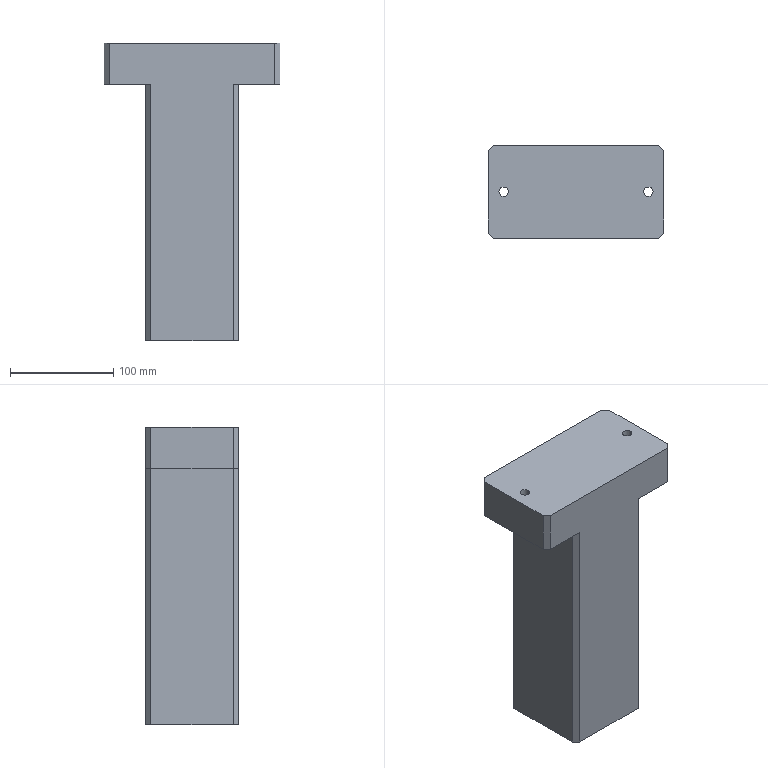Part | SolidWorks | features Chamfer 1, Extrusion 1, HoleWzd 1, ICE 1 | 1 solid | 22 faces | box 170 x 90 x 288 mm | volume 2601311 mm3 | plane 18 | cylinder 4 | commonest cylinder face diameters 9 x4
STEP:
#1=CARTESIAN_POINT('',(-65.5,0.,288.));
#2=VERTEX_POINT('',#1);
#3=CARTESIAN_POINT('',(-74.5,0.,288.));
#4=VERTEX_POINT('',#3);
#5=CARTESIAN_POINT('',(-70.,0.,288.));
#6=DIRECTION('',(0.,0.,-1.));
#7=DIRECTION('',(-1.,0.,0.));
#8=AXIS2_PLACEMENT_3D('',#5,#6,#7);
#9=CIRCLE('',#8,4.5);
#10=EDGE_CURVE('',#2,#4,#9,.T.);
#11=ORIENTED_EDGE('',*,*,#10,.F.);
#12=CARTESIAN_POINT('',(-65.5,0.,248.));
#13=VERTEX_POINT('',#12);
#14=CARTESIAN_POINT('',(-65.5,0.,248.));
#15=DIRECTION('',(0.,0.,-1.));
#16=VECTOR('',#15,1000.);
#17=LINE('',#14,#16);
#18=EDGE_CURVE('',#2,#13,#17,.T.);
#19=ORIENTED_EDGE('',*,*,#18,.T.);
#20=CARTESIAN_POINT('',(-74.5,0.,248.));
#21=VERTEX_POINT('',#20);
#22=CARTESIAN_POINT('',(-70.,0.,248.));
#23=DIRECTION('',(0.,0.,-1.));
#24=DIRECTION('',(-1.,0.,0.));
#25=AXIS2_PLACEMENT_3D('',#22,#23,#24);
#26=CIRCLE('',#25,4.5);
#27=EDGE_CURVE('',#13,#21,#26,.T.);
#28=ORIENTED_EDGE('',*,*,#27,.T.);
#29=CARTESIAN_POINT('',(-74.5,0.,248.));
#30=DIRECTION('',(0.,0.,-1.));
#31=VECTOR('',#30,1000.);
#32=LINE('',#29,#31);
#33=EDGE_CURVE('',#4,#21,#32,.T.);
#34=ORIENTED_EDGE('',*,*,#33,.F.);
#35=EDGE_LOOP('',(#11,#19,#28,#34));
#36=FACE_OUTER_BOUND('',#35,.T.);
#37=CARTESIAN_POINT('',(-70.,0.,248.));
#38=DIRECTION('',(0.,0.,-1.));
#39=DIRECTION('',(-1.,0.,0.));
#40=AXIS2_PLACEMENT_3D('',#37,#38,#39);
#41=CYLINDRICAL_SURFACE('',#40,4.5);
#42=ADVANCED_FACE('',(#36),#41,.F.);
#43=CARTESIAN_POINT('',(74.5,0.,288.));
#44=VERTEX_POINT('',#43);
#45=CARTESIAN_POINT('',(65.5,0.,288.));
#46=VERTEX_POINT('',#45);
#47=CARTESIAN_POINT('',(70.,0.,288.));
#48=DIRECTION('',(0.,0.,-1.));
#49=DIRECTION('',(-1.,0.,0.));
#50=AXIS2_PLACEMENT_3D('',#47,#48,#49);
#51=CIRCLE('',#50,4.5);
#52=EDGE_CURVE('',#44,#46,#51,.T.);
#53=ORIENTED_EDGE('',*,*,#52,.F.);
#54=CARTESIAN_POINT('',(74.5,0.,248.));
#55=VERTEX_POINT('',#54);
#56=CARTESIAN_POINT('',(74.5,0.,248.));
#57=DIRECTION('',(0.,0.,-1.));
#58=VECTOR('',#57,1000.);
#59=LINE('',#56,#58);
#60=EDGE_CURVE('',#44,#55,#59,.T.);
#61=ORIENTED_EDGE('',*,*,#60,.T.);
#62=CARTESIAN_POINT('',(65.5,0.,248.));
#63=VERTEX_POINT('',#62);
#64=CARTESIAN_POINT('',(70.,0.,248.));
#65=DIRECTION('',(0.,0.,-1.));
#66=DIRECTION('',(-1.,0.,0.));
#67=AXIS2_PLACEMENT_3D('',#64,#65,#66);
#68=CIRCLE('',#67,4.5);
#69=EDGE_CURVE('',#55,#63,#68,.T.);
#70=ORIENTED_EDGE('',*,*,#69,.T.);
#71=CARTESIAN_POINT('',(65.5,0.,248.));
#72=DIRECTION('',(0.,0.,-1.));
#73=VECTOR('',#72,1000.);
#74=LINE('',#71,#73);
#75=EDGE_CURVE('',#46,#63,#74,.T.);
#76=ORIENTED_EDGE('',*,*,#75,.F.);
#77=EDGE_LOOP('',(#53,#61,#70,#76));
#78=FACE_OUTER_BOUND('',#77,.T.);
#79=CARTESIAN_POINT('',(70.,0.,248.));
#80=DIRECTION('',(0.,0.,-1.));
#81=DIRECTION('',(-1.,0.,0.));
#82=AXIS2_PLACEMENT_3D('',#79,#80,#81);
#83=CYLINDRICAL_SURFACE('',#82,4.5);
#84=ADVANCED_FACE('',(#78),#83,.F.);
#85=CARTESIAN_POINT('',(45.,-40.,248.));
#86=VERTEX_POINT('',#85);
#87=CARTESIAN_POINT('',(45.,40.,248.));
#88=VERTEX_POINT('',#87);
#89=CARTESIAN_POINT('',(45.,45.,248.));
#90=DIRECTION('',(0.,1.,0.));
#91=VECTOR('',#90,1000.);
#92=LINE('',#89,#91);
#93=EDGE_CURVE('',#86,#88,#92,.T.);
#94=ORIENTED_EDGE('',*,*,#93,.F.);
#95=CARTESIAN_POINT('',(45.,-40.,0.));
#96=VERTEX_POINT('',#95);
#97=CARTESIAN_POINT('',(45.,-40.,288.));
#98=DIRECTION('',(0.,0.,-1.));
#99=VECTOR('',#98,1000.);
#100=LINE('',#97,#99);
#101=EDGE_CURVE('',#86,#96,#100,.T.);
#102=ORIENTED_EDGE('',*,*,#101,.T.);
#103=CARTESIAN_POINT('',(45.,40.,0.));
#104=VERTEX_POINT('',#103);
#105=CARTESIAN_POINT('',(45.,45.,0.));
#106=DIRECTION('',(0.,1.,0.));
#107=VECTOR('',#106,1000.);
#108=LINE('',#105,#107);
#109=EDGE_CURVE('',#96,#104,#108,.T.);
#110=ORIENTED_EDGE('',*,*,#109,.T.);
#111=CARTESIAN_POINT('',(45.,40.,288.));
#112=DIRECTION('',(0.,0.,1.));
#113=VECTOR('',#112,1000.);
#114=LINE('',#111,#113);
#115=EDGE_CURVE('',#104,#88,#114,.T.);
#116=ORIENTED_EDGE('',*,*,#115,.T.);
#117=EDGE_LOOP('',(#94,#102,#110,#116));
#118=FACE_OUTER_BOUND('',#117,.T.);
#119=CARTESIAN_POINT('',(45.,45.,288.));
#120=DIRECTION('',(-1.,0.,0.));
#121=DIRECTION('',(0.,-1.,0.));
#122=AXIS2_PLACEMENT_3D('',#119,#120,#121);
#123=PLANE('',#122);
#124=ADVANCED_FACE('',(#118),#123,.F.);
#125=CARTESIAN_POINT('',(-45.,40.,0.));
#126=VERTEX_POINT('',#125);
#127=CARTESIAN_POINT('',(-45.,-40.,0.));
#128=VERTEX_POINT('',#127);
#129=CARTESIAN_POINT('',(-45.,45.,0.));
#130=DIRECTION('',(0.,-1.,0.));
#131=VECTOR('',#130,1000.);
#132=LINE('',#129,#131);
#133=EDGE_CURVE('',#126,#128,#132,.T.);
#134=ORIENTED_EDGE('',*,*,#133,.T.);
#135=CARTESIAN_POINT('',(-45.,-40.,248.));
#136=VERTEX_POINT('',#135);
#137=CARTESIAN_POINT('',(-45.,-40.,288.));
#138=DIRECTION('',(0.,0.,1.));
#139=VECTOR('',#138,1000.);
#140=LINE('',#137,#139);
#141=EDGE_CURVE('',#128,#136,#140,.T.);
#142=ORIENTED_EDGE('',*,*,#141,.T.);
#143=CARTESIAN_POINT('',(-45.,40.,248.));
#144=VERTEX_POINT('',#143);
#145=CARTESIAN_POINT('',(-45.,45.,248.));
#146=DIRECTION('',(0.,-1.,0.));
#147=VECTOR('',#146,1000.);
#148=LINE('',#145,#147);
#149=EDGE_CURVE('',#144,#136,#148,.T.);
#150=ORIENTED_EDGE('',*,*,#149,.F.);
#151=CARTESIAN_POINT('',(-45.,40.,288.));
#152=DIRECTION('',(0.,0.,-1.));
#153=VECTOR('',#152,1000.);
#154=LINE('',#151,#153);
#155=EDGE_CURVE('',#144,#126,#154,.T.);
#156=ORIENTED_EDGE('',*,*,#155,.T.);
#157=EDGE_LOOP('',(#134,#142,#150,#156));
#158=FACE_OUTER_BOUND('',#157,.T.);
#159=CARTESIAN_POINT('',(-45.,45.,288.));
#160=DIRECTION('',(1.,0.,0.));
#161=DIRECTION('',(0.,1.,0.));
#162=AXIS2_PLACEMENT_3D('',#159,#160,#161);
#163=PLANE('',#162);
#164=ADVANCED_FACE('',(#158),#163,.F.);
#165=CARTESIAN_POINT('',(80.,45.,288.));
#166=VERTEX_POINT('',#165);
#167=CARTESIAN_POINT('',(-80.,45.,288.));
#168=VERTEX_POINT('',#167);
#169=CARTESIAN_POINT('',(-45.,45.,288.));
#170=DIRECTION('',(-1.,0.,0.));
#171=VECTOR('',#170,1000.);
#172=LINE('',#169,#171);
#173=EDGE_CURVE('',#166,#168,#172,.T.);
#174=ORIENTED_EDGE('',*,*,#173,.F.);
#175=CARTESIAN_POINT('',(80.,45.,248.));
#176=VERTEX_POINT('',#175);
#177=CARTESIAN_POINT('',(80.,45.,248.));
#178=DIRECTION('',(0.,0.,-1.));
#179=VECTOR('',#178,1000.);
#180=LINE('',#177,#179);
#181=EDGE_CURVE('',#166,#176,#180,.T.);
#182=ORIENTED_EDGE('',*,*,#181,.T.);
#183=CARTESIAN_POINT('',(40.,45.,248.));
#184=VERTEX_POINT('',#183);
#185=CARTESIAN_POINT('',(85.,45.,248.));
#186=DIRECTION('',(-1.,0.,0.));
#187=VECTOR('',#186,1000.);
#188=LINE('',#185,#187);
#189=EDGE_CURVE('',#176,#184,#188,.T.);
#190=ORIENTED_EDGE('',*,*,#189,.T.);
#191=CARTESIAN_POINT('',(40.,45.,0.));
#192=VERTEX_POINT('',#191);
#193=CARTESIAN_POINT('',(40.,45.,288.));
#194=DIRECTION('',(0.,0.,-1.));
#195=VECTOR('',#194,1000.);
#196=LINE('',#193,#195);
#197=EDGE_CURVE('',#184,#192,#196,.T.);
#198=ORIENTED_EDGE('',*,*,#197,.T.);
#199=CARTESIAN_POINT('',(-40.,45.,0.));
#200=VERTEX_POINT('',#199);
#201=CARTESIAN_POINT('',(-45.,45.,0.));
#202=DIRECTION('',(-1.,0.,0.));
#203=VECTOR('',#202,1000.);
#204=LINE('',#201,#203);
#205=EDGE_CURVE('',#192,#200,#204,.T.);
#206=ORIENTED_EDGE('',*,*,#205,.T.);
#207=CARTESIAN_POINT('',(-40.,45.,248.));
#208=VERTEX_POINT('',#207);
#209=CARTESIAN_POINT('',(-40.,45.,288.));
#210=DIRECTION('',(0.,0.,1.));
#211=VECTOR('',#210,1000.);
#212=LINE('',#209,#211);
#213=EDGE_CURVE('',#200,#208,#212,.T.);
#214=ORIENTED_EDGE('',*,*,#213,.T.);
#215=CARTESIAN_POINT('',(-80.,45.,248.));
#216=VERTEX_POINT('',#215);
#217=CARTESIAN_POINT('',(85.,45.,248.));
#218=DIRECTION('',(-1.,0.,0.));
#219=VECTOR('',#218,1000.);
#220=LINE('',#217,#219);
#221=EDGE_CURVE('',#208,#216,#220,.T.);
#222=ORIENTED_EDGE('',*,*,#221,.T.);
#223=CARTESIAN_POINT('',(-80.,45.,288.));
#224=DIRECTION('',(0.,0.,1.));
#225=VECTOR('',#224,1000.);
#226=LINE('',#223,#225);
#227=EDGE_CURVE('',#216,#168,#226,.T.);
#228=ORIENTED_EDGE('',*,*,#227,.T.);
#229=EDGE_LOOP('',(#174,#182,#190,#198,#206,#214,#222,#228));
#230=FACE_OUTER_BOUND('',#229,.T.);
#231=CARTESIAN_POINT('',(-45.,45.,288.));
#232=DIRECTION('',(0.,-1.,0.));
#233=DIRECTION('',(0.,0.,-1.));
#234=AXIS2_PLACEMENT_3D('',#231,#232,#233);
#235=PLANE('',#234);
#236=ADVANCED_FACE('',(#230),#235,.F.);
#237=CARTESIAN_POINT('',(40.,-45.,248.));
#238=VERTEX_POINT('',#237);
#239=CARTESIAN_POINT('',(80.,-45.,248.));
#240=VERTEX_POINT('',#239);
#241=CARTESIAN_POINT('',(85.,-45.,248.));
#242=DIRECTION('',(1.,0.,0.));
#243=VECTOR('',#242,1000.);
#244=LINE('',#241,#243);
#245=EDGE_CURVE('',#238,#240,#244,.T.);
#246=ORIENTED_EDGE('',*,*,#245,.T.);
#247=CARTESIAN_POINT('',(80.,-45.,288.));
#248=VERTEX_POINT('',#247);
#249=CARTESIAN_POINT('',(80.,-45.,288.));
#250=DIRECTION('',(0.,0.,1.));
#251=VECTOR('',#250,1000.);
#252=LINE('',#249,#251);
#253=EDGE_CURVE('',#240,#248,#252,.T.);
#254=ORIENTED_EDGE('',*,*,#253,.T.);
#255=CARTESIAN_POINT('',(-80.,-45.,288.));
#256=VERTEX_POINT('',#255);
#257=CARTESIAN_POINT('',(-45.,-45.,288.));
#258=DIRECTION('',(1.,0.,0.));
#259=VECTOR('',#258,1000.);
#260=LINE('',#257,#259);
#261=EDGE_CURVE('',#256,#248,#260,.T.);
#262=ORIENTED_EDGE('',*,*,#261,.F.);
#263=CARTESIAN_POINT('',(-80.,-45.,248.));
#264=VERTEX_POINT('',#263);
#265=CARTESIAN_POINT('',(-80.,-45.,248.));
#266=DIRECTION('',(0.,0.,-1.));
#267=VECTOR('',#266,1000.);
#268=LINE('',#265,#267);
#269=EDGE_CURVE('',#256,#264,#268,.T.);
#270=ORIENTED_EDGE('',*,*,#269,.T.);
#271=CARTESIAN_POINT('',(-40.,-45.,248.));
#272=VERTEX_POINT('',#271);
#273=CARTESIAN_POINT('',(85.,-45.,248.));
#274=DIRECTION('',(1.,0.,0.));
#275=VECTOR('',#274,1000.);
#276=LINE('',#273,#275);
#277=EDGE_CURVE('',#264,#272,#276,.T.);
#278=ORIENTED_EDGE('',*,*,#277,.T.);
#279=CARTESIAN_POINT('',(-40.,-45.,0.));
#280=VERTEX_POINT('',#279);
#281=CARTESIAN_POINT('',(-40.,-45.,288.));
#282=DIRECTION('',(0.,0.,-1.));
#283=VECTOR('',#282,1000.);
#284=LINE('',#281,#283);
#285=EDGE_CURVE('',#272,#280,#284,.T.);
#286=ORIENTED_EDGE('',*,*,#285,.T.);
#287=CARTESIAN_POINT('',(40.,-45.,0.));
#288=VERTEX_POINT('',#287);
#289=CARTESIAN_POINT('',(-45.,-45.,0.));
#290=DIRECTION('',(1.,0.,0.));
#291=VECTOR('',#290,1000.);
#292=LINE('',#289,#291);
#293=EDGE_CURVE('',#280,#288,#292,.T.);
#294=ORIENTED_EDGE('',*,*,#293,.T.);
#295=CARTESIAN_POINT('',(40.,-45.,288.));
#296=DIRECTION('',(0.,0.,1.));
#297=VECTOR('',#296,1000.);
#298=LINE('',#295,#297);
#299=EDGE_CURVE('',#288,#238,#298,.T.);
#300=ORIENTED_EDGE('',*,*,#299,.T.);
#301=EDGE_LOOP('',(#246,#254,#262,#270,#278,#286,#294,#300));
#302=FACE_OUTER_BOUND('',#301,.T.);
#303=CARTESIAN_POINT('',(-45.,-45.,288.));
#304=DIRECTION('',(0.,1.,0.));
#305=DIRECTION('',(0.,0.,1.));
#306=AXIS2_PLACEMENT_3D('',#303,#304,#305);
#307=PLANE('',#306);
#308=ADVANCED_FACE('',(#302),#307,.F.);
#309=CARTESIAN_POINT('',(-70.,0.,288.));
#310=DIRECTION('',(0.,0.,-1.));
#311=DIRECTION('',(-1.,0.,0.));
#312=AXIS2_PLACEMENT_3D('',#309,#310,#311);
#313=CIRCLE('',#312,4.5);
#314=EDGE_CURVE('',#4,#2,#313,.T.);
#315=ORIENTED_EDGE('',*,*,#314,.T.);
#316=ORIENTED_EDGE('',*,*,#10,.T.);
#317=EDGE_LOOP('',(#315,#316));
#318=FACE_BOUND('',#317,.T.);
#319=CARTESIAN_POINT('',(70.,0.,288.));
#320=DIRECTION('',(0.,0.,-1.));
#321=DIRECTION('',(-1.,0.,0.));
#322=AXIS2_PLACEMENT_3D('',#319,#320,#321);
#323=CIRCLE('',#322,4.5);
#324=EDGE_CURVE('',#46,#44,#323,.T.);
#325=ORIENTED_EDGE('',*,*,#324,.T.);
#326=ORIENTED_EDGE('',*,*,#52,.T.);
#327=EDGE_LOOP('',(#325,#326));
#328=FACE_BOUND('',#327,.T.);
#329=CARTESIAN_POINT('',(85.,-40.,288.));
#330=VERTEX_POINT('',#329);
#331=CARTESIAN_POINT('',(85.,40.,288.));
#332=VERTEX_POINT('',#331);
#333=CARTESIAN_POINT('',(85.,-45.,288.));
#334=DIRECTION('',(0.,1.,0.));
#335=VECTOR('',#334,1000.);
#336=LINE('',#333,#335);
#337=EDGE_CURVE('',#330,#332,#336,.T.);
#338=ORIENTED_EDGE('',*,*,#337,.T.);
#339=CARTESIAN_POINT('',(62.5,62.5,288.));
#340=DIRECTION('',(-0.7071,0.7071,0.));
#341=VECTOR('',#340,1000.);
#342=LINE('',#339,#341);
#343=EDGE_CURVE('',#332,#166,#342,.T.);
#344=ORIENTED_EDGE('',*,*,#343,.T.);
#345=ORIENTED_EDGE('',*,*,#173,.T.);
#346=CARTESIAN_POINT('',(-85.,40.,288.));
#347=VERTEX_POINT('',#346);
#348=CARTESIAN_POINT('',(-62.5,62.5,288.));
#349=DIRECTION('',(-0.7071,-0.7071,0.));
#350=VECTOR('',#349,1000.);
#351=LINE('',#348,#350);
#352=EDGE_CURVE('',#168,#347,#351,.T.);
#353=ORIENTED_EDGE('',*,*,#352,.T.);
#354=CARTESIAN_POINT('',(-85.,-40.,288.));
#355=VERTEX_POINT('',#354);
#356=CARTESIAN_POINT('',(-85.,-45.,288.));
#357=DIRECTION('',(0.,-1.,0.));
#358=VECTOR('',#357,1000.);
#359=LINE('',#356,#358);
#360=EDGE_CURVE('',#347,#355,#359,.T.);
#361=ORIENTED_EDGE('',*,*,#360,.T.);
#362=CARTESIAN_POINT('',(-62.5,-62.5,288.));
#363=DIRECTION('',(0.7071,-0.7071,0.));
#364=VECTOR('',#363,1000.);
#365=LINE('',#362,#364);
#366=EDGE_CURVE('',#355,#256,#365,.T.);
#367=ORIENTED_EDGE('',*,*,#366,.T.);
#368=ORIENTED_EDGE('',*,*,#261,.T.);
#369=CARTESIAN_POINT('',(62.5,-62.5,288.));
#370=DIRECTION('',(0.7071,0.7071,0.));
#371=VECTOR('',#370,1000.);
#372=LINE('',#369,#371);
#373=EDGE_CURVE('',#248,#330,#372,.T.);
#374=ORIENTED_EDGE('',*,*,#373,.T.);
#375=EDGE_LOOP('',(#338,#344,#345,#353,#361,#367,#368,#374));
#376=FACE_OUTER_BOUND('',#375,.T.);
#377=CARTESIAN_POINT('',(0.,0.,288.));
#378=DIRECTION('',(0.,0.,1.));
#379=DIRECTION('',(1.,0.,0.));
#380=AXIS2_PLACEMENT_3D('',#377,#378,#379);
#381=PLANE('',#380);
#382=ADVANCED_FACE('',(#318,#328,#376),#381,.T.);
#383=ORIENTED_EDGE('',*,*,#293,.F.);
#384=CARTESIAN_POINT('',(-40.,-45.,0.));
#385=DIRECTION('',(-0.7071,0.7071,0.));
#386=VECTOR('',#385,1000.);
#387=LINE('',#384,#386);
#388=EDGE_CURVE('',#280,#128,#387,.T.);
#389=ORIENTED_EDGE('',*,*,#388,.T.);
#390=ORIENTED_EDGE('',*,*,#133,.F.);
#391=CARTESIAN_POINT('',(-45.,40.,0.));
#392=DIRECTION('',(0.7071,0.7071,0.));
#393=VECTOR('',#392,1000.);
#394=LINE('',#391,#393);
#395=EDGE_CURVE('',#126,#200,#394,.T.);
#396=ORIENTED_EDGE('',*,*,#395,.T.);
#397=ORIENTED_EDGE('',*,*,#205,.F.);
#398=CARTESIAN_POINT('',(40.,45.,0.));
#399=DIRECTION('',(0.7071,-0.7071,0.));
#400=VECTOR('',#399,1000.);
#401=LINE('',#398,#400);
#402=EDGE_CURVE('',#192,#104,#401,.T.);
#403=ORIENTED_EDGE('',*,*,#402,.T.);
#404=ORIENTED_EDGE('',*,*,#109,.F.);
#405=CARTESIAN_POINT('',(45.,-40.,0.));
#406=DIRECTION('',(-0.7071,-0.7071,0.));
#407=VECTOR('',#406,1000.);
#408=LINE('',#405,#407);
#409=EDGE_CURVE('',#96,#288,#408,.T.);
#410=ORIENTED_EDGE('',*,*,#409,.T.);
#411=EDGE_LOOP('',(#383,#389,#390,#396,#397,#403,#404,#410));
#412=FACE_OUTER_BOUND('',#411,.T.);
#413=CARTESIAN_POINT('',(0.,0.,0.));
#414=DIRECTION('',(0.,0.,1.));
#415=DIRECTION('',(1.,0.,0.));
#416=AXIS2_PLACEMENT_3D('',#413,#414,#415);
#417=PLANE('',#416);
#418=ADVANCED_FACE('',(#412),#417,.F.);
#419=ORIENTED_EDGE('',*,*,#360,.F.);
#420=CARTESIAN_POINT('',(-85.,40.,248.));
#421=VERTEX_POINT('',#420);
#422=CARTESIAN_POINT('',(-85.,40.,248.));
#423=DIRECTION('',(0.,0.,-1.));
#424=VECTOR('',#423,1000.);
#425=LINE('',#422,#424);
#426=EDGE_CURVE('',#347,#421,#425,.T.);
#427=ORIENTED_EDGE('',*,*,#426,.T.);
#428=CARTESIAN_POINT('',(-85.,-40.,248.));
#429=VERTEX_POINT('',#428);
#430=CARTESIAN_POINT('',(-85.,-45.,248.));
#431=DIRECTION('',(0.,-1.,0.));
#432=VECTOR('',#431,1000.);
#433=LINE('',#430,#432);
#434=EDGE_CURVE('',#421,#429,#433,.T.);
#435=ORIENTED_EDGE('',*,*,#434,.T.);
#436=CARTESIAN_POINT('',(-85.,-40.,288.));
#437=DIRECTION('',(0.,0.,1.));
#438=VECTOR('',#437,1000.);
#439=LINE('',#436,#438);
#440=EDGE_CURVE('',#429,#355,#439,.T.);
#441=ORIENTED_EDGE('',*,*,#440,.T.);
#442=EDGE_LOOP('',(#419,#427,#435,#441));
#443=FACE_OUTER_BOUND('',#442,.T.);
#444=CARTESIAN_POINT('',(-85.,-45.,248.));
#445=DIRECTION('',(-1.,0.,0.));
#446=DIRECTION('',(0.,0.,1.));
#447=AXIS2_PLACEMENT_3D('',#444,#445,#446);
#448=PLANE('',#447);
#449=ADVANCED_FACE('',(#443),#448,.T.);
#450=CARTESIAN_POINT('',(-70.,0.,248.));
#451=DIRECTION('',(0.,0.,-1.));
#452=DIRECTION('',(-1.,0.,0.));
#453=AXIS2_PLACEMENT_3D('',#450,#451,#452);
#454=CIRCLE('',#453,4.5);
#455=EDGE_CURVE('',#21,#13,#454,.T.);
#456=ORIENTED_EDGE('',*,*,#455,.F.);
#457=ORIENTED_EDGE('',*,*,#27,.F.);
#458=EDGE_LOOP('',(#456,#457));
#459=FACE_BOUND('',#458,.T.);
#460=ORIENTED_EDGE('',*,*,#434,.F.);
#461=CARTESIAN_POINT('',(-80.,45.,248.));
#462=DIRECTION('',(0.7071,0.7071,0.));
#463=VECTOR('',#462,1000.);
#464=LINE('',#461,#463);
#465=EDGE_CURVE('',#421,#216,#464,.T.);
#466=ORIENTED_EDGE('',*,*,#465,.T.);
#467=ORIENTED_EDGE('',*,*,#221,.F.);
#468=CARTESIAN_POINT('',(-42.5,42.5,248.));
#469=DIRECTION('',(-0.7071,-0.7071,0.));
#470=VECTOR('',#469,1000.);
#471=LINE('',#468,#470);
#472=EDGE_CURVE('',#208,#144,#471,.T.);
#473=ORIENTED_EDGE('',*,*,#472,.T.);
#474=ORIENTED_EDGE('',*,*,#149,.T.);
#475=CARTESIAN_POINT('',(-42.5,-42.5,248.));
#476=DIRECTION('',(0.7071,-0.7071,0.));
#477=VECTOR('',#476,1000.);
#478=LINE('',#475,#477);
#479=EDGE_CURVE('',#136,#272,#478,.T.);
#480=ORIENTED_EDGE('',*,*,#479,.T.);
#481=ORIENTED_EDGE('',*,*,#277,.F.);
#482=CARTESIAN_POINT('',(-85.,-40.,248.));
#483=DIRECTION('',(-0.7071,0.7071,0.));
#484=VECTOR('',#483,1000.);
#485=LINE('',#482,#484);
#486=EDGE_CURVE('',#264,#429,#485,.T.);
#487=ORIENTED_EDGE('',*,*,#486,.T.);
#488=EDGE_LOOP('',(#460,#466,#467,#473,#474,#480,#481,#487));
#489=FACE_OUTER_BOUND('',#488,.T.);
#490=CARTESIAN_POINT('',(0.,0.,248.));
#491=DIRECTION('',(0.,0.,1.));
#492=DIRECTION('',(1.,0.,0.));
#493=AXIS2_PLACEMENT_3D('',#490,#491,#492);
#494=PLANE('',#493);
#495=ADVANCED_FACE('',(#459,#489),#494,.F.);
#496=CARTESIAN_POINT('',(70.,0.,248.));
#497=DIRECTION('',(0.,0.,-1.));
#498=DIRECTION('',(-1.,0.,0.));
#499=AXIS2_PLACEMENT_3D('',#496,#497,#498);
#500=CIRCLE('',#499,4.5);
#501=EDGE_CURVE('',#63,#55,#500,.T.);
#502=ORIENTED_EDGE('',*,*,#501,.F.);
#503=ORIENTED_EDGE('',*,*,#69,.F.);
#504=EDGE_LOOP('',(#502,#503));
#505=FACE_BOUND('',#504,.T.);
#506=ORIENTED_EDGE('',*,*,#189,.F.);
#507=CARTESIAN_POINT('',(85.,40.,248.));
#508=VERTEX_POINT('',#507);
#509=CARTESIAN_POINT('',(85.,40.,248.));
#510=DIRECTION('',(0.7071,-0.7071,0.));
#511=VECTOR('',#510,1000.);
#512=LINE('',#509,#511);
#513=EDGE_CURVE('',#176,#508,#512,.T.);
#514=ORIENTED_EDGE('',*,*,#513,.T.);
#515=CARTESIAN_POINT('',(85.,-40.,248.));
#516=VERTEX_POINT('',#515);
#517=CARTESIAN_POINT('',(85.,-45.,248.));
#518=DIRECTION('',(0.,1.,0.));
#519=VECTOR('',#518,1000.);
#520=LINE('',#517,#519);
#521=EDGE_CURVE('',#516,#508,#520,.T.);
#522=ORIENTED_EDGE('',*,*,#521,.F.);
#523=CARTESIAN_POINT('',(80.,-45.,248.));
#524=DIRECTION('',(-0.7071,-0.7071,0.));
#525=VECTOR('',#524,1000.);
#526=LINE('',#523,#525);
#527=EDGE_CURVE('',#516,#240,#526,.T.);
#528=ORIENTED_EDGE('',*,*,#527,.T.);
#529=ORIENTED_EDGE('',*,*,#245,.F.);
#530=CARTESIAN_POINT('',(42.5,-42.5,248.));
#531=DIRECTION('',(0.7071,0.7071,0.));
#532=VECTOR('',#531,1000.);
#533=LINE('',#530,#532);
#534=EDGE_CURVE('',#238,#86,#533,.T.);
#535=ORIENTED_EDGE('',*,*,#534,.T.);
#536=ORIENTED_EDGE('',*,*,#93,.T.);
#537=CARTESIAN_POINT('',(42.5,42.5,248.));
#538=DIRECTION('',(-0.7071,0.7071,0.));
#539=VECTOR('',#538,1000.);
#540=LINE('',#537,#539);
#541=EDGE_CURVE('',#88,#184,#540,.T.);
#542=ORIENTED_EDGE('',*,*,#541,.T.);
#543=EDGE_LOOP('',(#506,#514,#522,#528,#529,#535,#536,#542));
#544=FACE_OUTER_BOUND('',#543,.T.);
#545=CARTESIAN_POINT('',(0.,0.,248.));
#546=DIRECTION('',(0.,0.,1.));
#547=DIRECTION('',(1.,0.,0.));
#548=AXIS2_PLACEMENT_3D('',#545,#546,#547);
#549=PLANE('',#548);
#550=ADVANCED_FACE('',(#505,#544),#549,.F.);
#551=ORIENTED_EDGE('',*,*,#521,.T.);
#552=CARTESIAN_POINT('',(85.,40.,288.));
#553=DIRECTION('',(0.,0.,1.));
#554=VECTOR('',#553,1000.);
#555=LINE('',#552,#554);
#556=EDGE_CURVE('',#508,#332,#555,.T.);
#557=ORIENTED_EDGE('',*,*,#556,.T.);
#558=ORIENTED_EDGE('',*,*,#337,.F.);
#559=CARTESIAN_POINT('',(85.,-40.,248.));
#560=DIRECTION('',(0.,0.,-1.));
#561=VECTOR('',#560,1000.);
#562=LINE('',#559,#561);
#563=EDGE_CURVE('',#330,#516,#562,.T.);
#564=ORIENTED_EDGE('',*,*,#563,.T.);
#565=EDGE_LOOP('',(#551,#557,#558,#564));
#566=FACE_OUTER_BOUND('',#565,.T.);
#567=CARTESIAN_POINT('',(85.,-45.,248.));
#568=DIRECTION('',(1.,0.,0.));
#569=DIRECTION('',(0.,0.,-1.));
#570=AXIS2_PLACEMENT_3D('',#567,#568,#569);
#571=PLANE('',#570);
#572=ADVANCED_FACE('',(#566),#571,.T.);
#573=ORIENTED_EDGE('',*,*,#513,.F.);
#574=ORIENTED_EDGE('',*,*,#181,.F.);
#575=ORIENTED_EDGE('',*,*,#343,.F.);
#576=ORIENTED_EDGE('',*,*,#556,.F.);
#577=EDGE_LOOP('',(#573,#574,#575,#576));
#578=FACE_OUTER_BOUND('',#577,.T.);
#579=CARTESIAN_POINT('',(85.,40.,248.));
#580=DIRECTION('',(0.7071,0.7071,0.));
#581=DIRECTION('',(0.,0.,-1.));
#582=AXIS2_PLACEMENT_3D('',#579,#580,#581);
#583=PLANE('',#582);
#584=ADVANCED_FACE('',(#578),#583,.T.);
#585=ORIENTED_EDGE('',*,*,#527,.F.);
#586=ORIENTED_EDGE('',*,*,#563,.F.);
#587=ORIENTED_EDGE('',*,*,#373,.F.);
#588=ORIENTED_EDGE('',*,*,#253,.F.);
#589=EDGE_LOOP('',(#585,#586,#587,#588));
#590=FACE_OUTER_BOUND('',#589,.T.);
#591=CARTESIAN_POINT('',(80.,-45.,288.));
#592=DIRECTION('',(0.7071,-0.7071,0.));
#593=DIRECTION('',(0.,0.,-1.));
#594=AXIS2_PLACEMENT_3D('',#591,#592,#593);
#595=PLANE('',#594);
#596=ADVANCED_FACE('',(#590),#595,.T.);
#597=ORIENTED_EDGE('',*,*,#465,.F.);
#598=ORIENTED_EDGE('',*,*,#426,.F.);
#599=ORIENTED_EDGE('',*,*,#352,.F.);
#600=ORIENTED_EDGE('',*,*,#227,.F.);
#601=EDGE_LOOP('',(#597,#598,#599,#600));
#602=FACE_OUTER_BOUND('',#601,.T.);
#603=CARTESIAN_POINT('',(-80.,45.,288.));
#604=DIRECTION('',(-0.7071,0.7071,0.));
#605=DIRECTION('',(0.,0.,-1.));
#606=AXIS2_PLACEMENT_3D('',#603,#604,#605);
#607=PLANE('',#606);
#608=ADVANCED_FACE('',(#602),#607,.T.);
#609=ORIENTED_EDGE('',*,*,#486,.F.);
#610=ORIENTED_EDGE('',*,*,#269,.F.);
#611=ORIENTED_EDGE('',*,*,#366,.F.);
#612=ORIENTED_EDGE('',*,*,#440,.F.);
#613=EDGE_LOOP('',(#609,#610,#611,#612));
#614=FACE_OUTER_BOUND('',#613,.T.);
#615=CARTESIAN_POINT('',(-85.,-40.,248.));
#616=DIRECTION('',(-0.7071,-0.7071,0.));
#617=DIRECTION('',(0.,0.,-1.));
#618=AXIS2_PLACEMENT_3D('',#615,#616,#617);
#619=PLANE('',#618);
#620=ADVANCED_FACE('',(#614),#619,.T.);
#621=ORIENTED_EDGE('',*,*,#479,.F.);
#622=ORIENTED_EDGE('',*,*,#141,.F.);
#623=ORIENTED_EDGE('',*,*,#388,.F.);
#624=ORIENTED_EDGE('',*,*,#285,.F.);
#625=EDGE_LOOP('',(#621,#622,#623,#624));
#626=FACE_OUTER_BOUND('',#625,.T.);
#627=CARTESIAN_POINT('',(-40.,-45.,288.));
#628=DIRECTION('',(0.7071,0.7071,0.));
#629=DIRECTION('',(0.,0.,-1.));
#630=AXIS2_PLACEMENT_3D('',#627,#628,#629);
#631=PLANE('',#630);
#632=ADVANCED_FACE('',(#626),#631,.F.);
#633=ORIENTED_EDGE('',*,*,#472,.F.);
#634=ORIENTED_EDGE('',*,*,#213,.F.);
#635=ORIENTED_EDGE('',*,*,#395,.F.);
#636=ORIENTED_EDGE('',*,*,#155,.F.);
#637=EDGE_LOOP('',(#633,#634,#635,#636));
#638=FACE_OUTER_BOUND('',#637,.T.);
#639=CARTESIAN_POINT('',(-45.,40.,288.));
#640=DIRECTION('',(0.7071,-0.7071,0.));
#641=DIRECTION('',(0.,0.,-1.));
#642=AXIS2_PLACEMENT_3D('',#639,#640,#641);
#643=PLANE('',#642);
#644=ADVANCED_FACE('',(#638),#643,.F.);
#645=ORIENTED_EDGE('',*,*,#534,.F.);
#646=ORIENTED_EDGE('',*,*,#299,.F.);
#647=ORIENTED_EDGE('',*,*,#409,.F.);
#648=ORIENTED_EDGE('',*,*,#101,.F.);
#649=EDGE_LOOP('',(#645,#646,#647,#648));
#650=FACE_OUTER_BOUND('',#649,.T.);
#651=CARTESIAN_POINT('',(45.,-40.,288.));
#652=DIRECTION('',(-0.7071,0.7071,0.));
#653=DIRECTION('',(0.,0.,-1.));
#654=AXIS2_PLACEMENT_3D('',#651,#652,#653);
#655=PLANE('',#654);
#656=ADVANCED_FACE('',(#650),#655,.F.);
#657=ORIENTED_EDGE('',*,*,#541,.F.);
#658=ORIENTED_EDGE('',*,*,#115,.F.);
#659=ORIENTED_EDGE('',*,*,#402,.F.);
#660=ORIENTED_EDGE('',*,*,#197,.F.);
#661=EDGE_LOOP('',(#657,#658,#659,#660));
#662=FACE_OUTER_BOUND('',#661,.T.);
#663=CARTESIAN_POINT('',(40.,45.,288.));
#664=DIRECTION('',(-0.7071,-0.7071,0.));
#665=DIRECTION('',(0.,0.,-1.));
#666=AXIS2_PLACEMENT_3D('',#663,#664,#665);
#667=PLANE('',#666);
#668=ADVANCED_FACE('',(#662),#667,.F.);
#669=ORIENTED_EDGE('',*,*,#60,.F.);
#670=ORIENTED_EDGE('',*,*,#324,.F.);
#671=ORIENTED_EDGE('',*,*,#75,.T.);
#672=ORIENTED_EDGE('',*,*,#501,.T.);
#673=EDGE_LOOP('',(#669,#670,#671,#672));
#674=FACE_OUTER_BOUND('',#673,.T.);
#675=CARTESIAN_POINT('',(70.,0.,248.));
#676=DIRECTION('',(0.,0.,-1.));
#677=DIRECTION('',(-1.,0.,0.));
#678=AXIS2_PLACEMENT_3D('',#675,#676,#677);
#679=CYLINDRICAL_SURFACE('',#678,4.5);
#680=ADVANCED_FACE('',(#674),#679,.F.);
#681=ORIENTED_EDGE('',*,*,#18,.F.);
#682=ORIENTED_EDGE('',*,*,#314,.F.);
#683=ORIENTED_EDGE('',*,*,#33,.T.);
#684=ORIENTED_EDGE('',*,*,#455,.T.);
#685=EDGE_LOOP('',(#681,#682,#683,#684));
#686=FACE_OUTER_BOUND('',#685,.T.);
#687=CARTESIAN_POINT('',(-70.,0.,248.));
#688=DIRECTION('',(0.,0.,-1.));
#689=DIRECTION('',(-1.,0.,0.));
#690=AXIS2_PLACEMENT_3D('',#687,#688,#689);
#691=CYLINDRICAL_SURFACE('',#690,4.5);
#692=ADVANCED_FACE('',(#686),#691,.F.);
#693=CLOSED_SHELL('',(#42,#84,#124,#164,#236,#308,#382,#418,#449,#495,#550,#572,#584,#596,#608,#620,#632,#644,#656,#668,#680,#692));
#694=MANIFOLD_SOLID_BREP('',#693);
#695=CARTESIAN_POINT('',(0.,0.,0.));
#696=DIRECTION('',(0.,0.,1.));
#697=DIRECTION('',(1.,0.,0.));
#698=AXIS2_PLACEMENT_3D('',#695,#696,#697);
#699=(LENGTH_UNIT()NAMED_UNIT(*)SI_UNIT(.MILLI.,.METRE.));
#700=UNCERTAINTY_MEASURE_WITH_UNIT(LENGTH_MEASURE(0.00001),#699,'','');
#701=(NAMED_UNIT(*)PLANE_ANGLE_UNIT()SI_UNIT($,.RADIAN.));
#702=(NAMED_UNIT(*)SI_UNIT($,.STERADIAN.)SOLID_ANGLE_UNIT());
#703=(GEOMETRIC_REPRESENTATION_CONTEXT(3)GLOBAL_UNCERTAINTY_ASSIGNED_CONTEXT((#700))GLOBAL_UNIT_ASSIGNED_CONTEXT((#699,#701,#702))REPRESENTATION_CONTEXT('',''));
#704=ADVANCED_BREP_SHAPE_REPRESENTATION('',(#694,#698),#703);